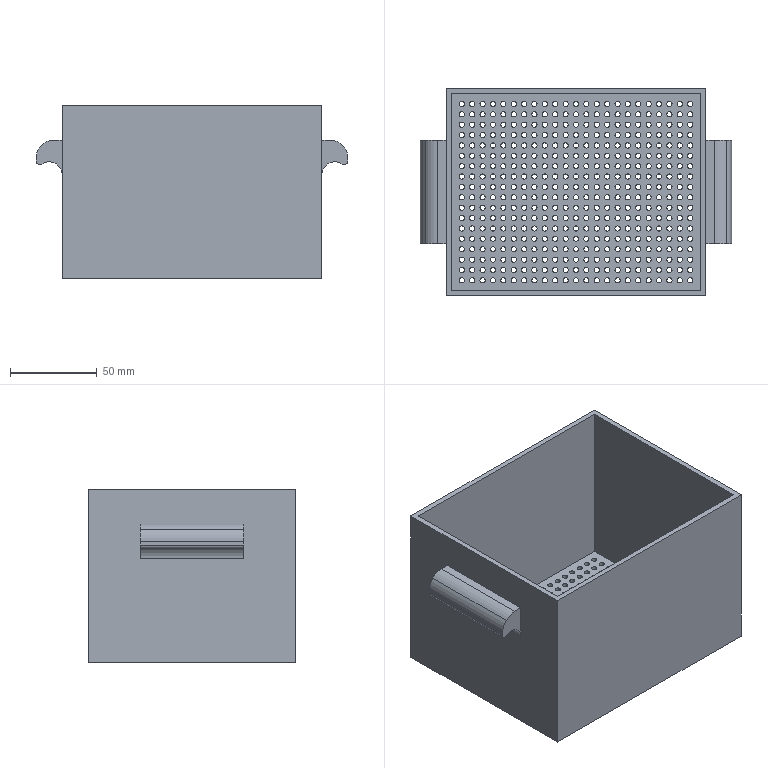Part | SolidWorks | features BaseBody 1 | 1 solid | 857 faces | box 180 x 120 x 100 mm | volume 221018 mm3 | cylinder 838 | plane 19 | commonest cylinder face diameters 3 x828 4 x4 20 x4 15 x2